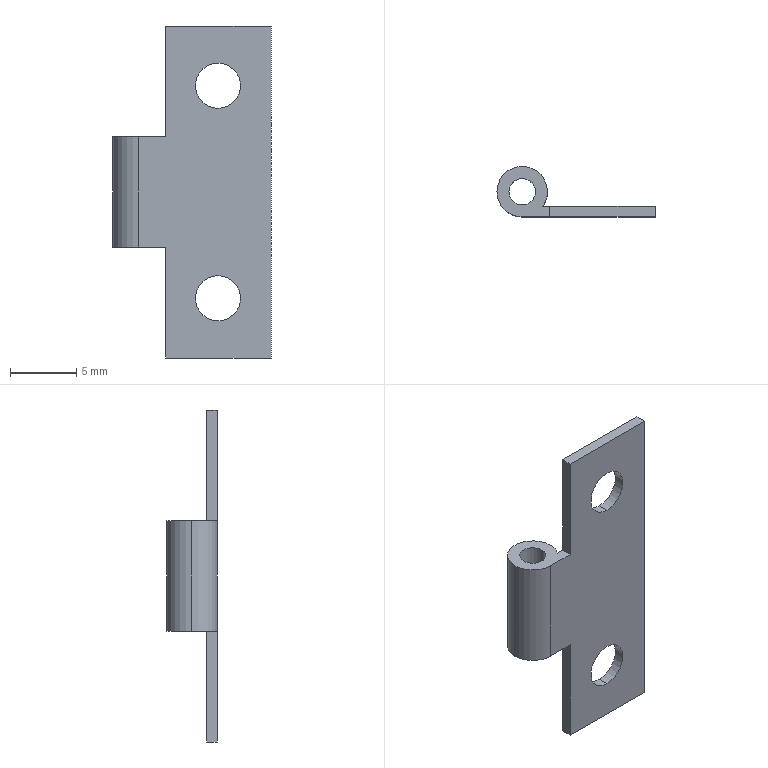Part | SolidWorks | features ICE 3, RefAxis 3, 3DProfileFeature 1, Extrusion 1 | 1 solid | 18 faces | box 11.9 x 3.8 x 25 mm | volume 218.697 mm3 | cylinder 9 | plane 9 | commonest cylinder face diameters 3.4 x4 3.8 x3 2 x2
STEP:
#1=CARTESIAN_POINT('',(6.,0.8,-6.2));
#2=VERTEX_POINT('',#1);
#3=CARTESIAN_POINT('',(6.,0.8,-2.8));
#4=VERTEX_POINT('',#3);
#5=CARTESIAN_POINT('',(6.,0.8,-4.5));
#6=DIRECTION('',(0.,1.,0.));
#7=DIRECTION('',(0.,0.,1.));
#8=AXIS2_PLACEMENT_3D('',#5,#6,#7);
#9=CIRCLE('',#8,1.7);
#10=EDGE_CURVE('',#2,#4,#9,.T.);
#11=ORIENTED_EDGE('',*,*,#10,.T.);
#12=CARTESIAN_POINT('',(6.,0.,-2.8));
#13=VERTEX_POINT('',#12);
#14=CARTESIAN_POINT('',(6.,0.8,-2.8));
#15=DIRECTION('',(0.,-1.,0.));
#16=VECTOR('',#15,1000.);
#17=LINE('',#14,#16);
#18=EDGE_CURVE('',#4,#13,#17,.T.);
#19=ORIENTED_EDGE('',*,*,#18,.T.);
#20=CARTESIAN_POINT('',(6.,0.,-6.2));
#21=VERTEX_POINT('',#20);
#22=CARTESIAN_POINT('',(6.,0.,-4.5));
#23=DIRECTION('',(0.,1.,0.));
#24=DIRECTION('',(0.,0.,1.));
#25=AXIS2_PLACEMENT_3D('',#22,#23,#24);
#26=CIRCLE('',#25,1.7);
#27=EDGE_CURVE('',#21,#13,#26,.T.);
#28=ORIENTED_EDGE('',*,*,#27,.F.);
#29=CARTESIAN_POINT('',(6.,0.8,-6.2));
#30=DIRECTION('',(0.,-1.,0.));
#31=VECTOR('',#30,1000.);
#32=LINE('',#29,#31);
#33=EDGE_CURVE('',#2,#21,#32,.T.);
#34=ORIENTED_EDGE('',*,*,#33,.F.);
#35=EDGE_LOOP('',(#11,#19,#28,#34));
#36=FACE_OUTER_BOUND('',#35,.T.);
#37=CARTESIAN_POINT('',(6.,0.8,-4.5));
#38=DIRECTION('',(0.,-1.,0.));
#39=DIRECTION('',(0.,0.,-1.));
#40=AXIS2_PLACEMENT_3D('',#37,#38,#39);
#41=CYLINDRICAL_SURFACE('',#40,1.7);
#42=ADVANCED_FACE('',(#36),#41,.F.);
#43=CARTESIAN_POINT('',(6.,0.8,-22.2));
#44=VERTEX_POINT('',#43);
#45=CARTESIAN_POINT('',(6.,0.8,-18.8));
#46=VERTEX_POINT('',#45);
#47=CARTESIAN_POINT('',(6.,0.8,-20.5));
#48=DIRECTION('',(0.,1.,0.));
#49=DIRECTION('',(0.,0.,1.));
#50=AXIS2_PLACEMENT_3D('',#47,#48,#49);
#51=CIRCLE('',#50,1.7);
#52=EDGE_CURVE('',#44,#46,#51,.T.);
#53=ORIENTED_EDGE('',*,*,#52,.T.);
#54=CARTESIAN_POINT('',(6.,0.,-18.8));
#55=VERTEX_POINT('',#54);
#56=CARTESIAN_POINT('',(6.,0.8,-18.8));
#57=DIRECTION('',(0.,-1.,0.));
#58=VECTOR('',#57,1000.);
#59=LINE('',#56,#58);
#60=EDGE_CURVE('',#46,#55,#59,.T.);
#61=ORIENTED_EDGE('',*,*,#60,.T.);
#62=CARTESIAN_POINT('',(6.,0.,-22.2));
#63=VERTEX_POINT('',#62);
#64=CARTESIAN_POINT('',(6.,0.,-20.5));
#65=DIRECTION('',(0.,1.,0.));
#66=DIRECTION('',(0.,0.,1.));
#67=AXIS2_PLACEMENT_3D('',#64,#65,#66);
#68=CIRCLE('',#67,1.7);
#69=EDGE_CURVE('',#63,#55,#68,.T.);
#70=ORIENTED_EDGE('',*,*,#69,.F.);
#71=CARTESIAN_POINT('',(6.,0.8,-22.2));
#72=DIRECTION('',(0.,-1.,0.));
#73=VECTOR('',#72,1000.);
#74=LINE('',#71,#73);
#75=EDGE_CURVE('',#44,#63,#74,.T.);
#76=ORIENTED_EDGE('',*,*,#75,.F.);
#77=EDGE_LOOP('',(#53,#61,#70,#76));
#78=FACE_OUTER_BOUND('',#77,.T.);
#79=CARTESIAN_POINT('',(6.,0.8,-20.5));
#80=DIRECTION('',(0.,-1.,0.));
#81=DIRECTION('',(0.,0.,-1.));
#82=AXIS2_PLACEMENT_3D('',#79,#80,#81);
#83=CYLINDRICAL_SURFACE('',#82,1.7);
#84=ADVANCED_FACE('',(#78),#83,.F.);
#85=CARTESIAN_POINT('',(-1.,1.9,-16.667));
#86=VERTEX_POINT('',#85);
#87=CARTESIAN_POINT('',(1.,1.9,-16.667));
#88=VERTEX_POINT('',#87);
#89=CARTESIAN_POINT('',(0.,1.9,-16.667));
#90=DIRECTION('',(0.,0.,1.));
#91=DIRECTION('',(-1.,0.,0.));
#92=AXIS2_PLACEMENT_3D('',#89,#90,#91);
#93=CIRCLE('',#92,1.);
#94=EDGE_CURVE('',#86,#88,#93,.T.);
#95=ORIENTED_EDGE('',*,*,#94,.F.);
#96=CARTESIAN_POINT('',(-1.,1.9,-8.333));
#97=VERTEX_POINT('',#96);
#98=CARTESIAN_POINT('',(-1.,1.9,-25.));
#99=DIRECTION('',(0.,0.,1.));
#100=VECTOR('',#99,1000.);
#101=LINE('',#98,#100);
#102=EDGE_CURVE('',#86,#97,#101,.T.);
#103=ORIENTED_EDGE('',*,*,#102,.T.);
#104=CARTESIAN_POINT('',(1.,1.9,-8.333));
#105=VERTEX_POINT('',#104);
#106=CARTESIAN_POINT('',(0.,1.9,-8.333));
#107=DIRECTION('',(0.,0.,-1.));
#108=DIRECTION('',(1.,0.,0.));
#109=AXIS2_PLACEMENT_3D('',#106,#107,#108);
#110=CIRCLE('',#109,1.);
#111=EDGE_CURVE('',#105,#97,#110,.T.);
#112=ORIENTED_EDGE('',*,*,#111,.F.);
#113=CARTESIAN_POINT('',(1.,1.9,-25.));
#114=DIRECTION('',(0.,0.,1.));
#115=VECTOR('',#114,1000.);
#116=LINE('',#113,#115);
#117=EDGE_CURVE('',#88,#105,#116,.T.);
#118=ORIENTED_EDGE('',*,*,#117,.F.);
#119=EDGE_LOOP('',(#95,#103,#112,#118));
#120=FACE_OUTER_BOUND('',#119,.T.);
#121=CARTESIAN_POINT('',(0.,1.9,-25.));
#122=DIRECTION('',(0.,0.,1.));
#123=DIRECTION('',(1.,0.,0.));
#124=AXIS2_PLACEMENT_3D('',#121,#122,#123);
#125=CYLINDRICAL_SURFACE('',#124,1.);
#126=ADVANCED_FACE('',(#120),#125,.F.);
#127=CARTESIAN_POINT('',(1.9,1.9,-16.667));
#128=VERTEX_POINT('',#127);
#129=CARTESIAN_POINT('',(-1.9,1.9,-16.667));
#130=VERTEX_POINT('',#129);
#131=CARTESIAN_POINT('',(0.,1.9,-16.667));
#132=DIRECTION('',(0.,0.,1.));
#133=DIRECTION('',(-1.,0.,0.));
#134=AXIS2_PLACEMENT_3D('',#131,#132,#133);
#135=CIRCLE('',#134,1.9);
#136=EDGE_CURVE('',#128,#130,#135,.T.);
#137=ORIENTED_EDGE('',*,*,#136,.T.);
#138=CARTESIAN_POINT('',(-1.9,1.9,-8.333));
#139=VERTEX_POINT('',#138);
#140=CARTESIAN_POINT('',(-1.9,1.9,-25.));
#141=DIRECTION('',(0.,0.,1.));
#142=VECTOR('',#141,1000.);
#143=LINE('',#140,#142);
#144=EDGE_CURVE('',#130,#139,#143,.T.);
#145=ORIENTED_EDGE('',*,*,#144,.T.);
#146=CARTESIAN_POINT('',(1.9,1.9,-8.333));
#147=VERTEX_POINT('',#146);
#148=CARTESIAN_POINT('',(0.,1.9,-8.333));
#149=DIRECTION('',(0.,0.,-1.));
#150=DIRECTION('',(1.,0.,0.));
#151=AXIS2_PLACEMENT_3D('',#148,#149,#150);
#152=CIRCLE('',#151,1.9);
#153=EDGE_CURVE('',#139,#147,#152,.T.);
#154=ORIENTED_EDGE('',*,*,#153,.T.);
#155=CARTESIAN_POINT('',(1.9,1.9,-25.));
#156=DIRECTION('',(0.,0.,1.));
#157=VECTOR('',#156,1000.);
#158=LINE('',#155,#157);
#159=EDGE_CURVE('',#128,#147,#158,.T.);
#160=ORIENTED_EDGE('',*,*,#159,.F.);
#161=EDGE_LOOP('',(#137,#145,#154,#160));
#162=FACE_OUTER_BOUND('',#161,.T.);
#163=CARTESIAN_POINT('',(0.,1.9,-25.));
#164=DIRECTION('',(0.,0.,1.));
#165=DIRECTION('',(1.,0.,0.));
#166=AXIS2_PLACEMENT_3D('',#163,#164,#165);
#167=CYLINDRICAL_SURFACE('',#166,1.9);
#168=ADVANCED_FACE('',(#162),#167,.T.);
#169=CARTESIAN_POINT('',(1.549,0.8,-16.667));
#170=VERTEX_POINT('',#169);
#171=CARTESIAN_POINT('',(0.,1.9,-16.667));
#172=DIRECTION('',(0.,0.,1.));
#173=DIRECTION('',(-1.,0.,0.));
#174=AXIS2_PLACEMENT_3D('',#171,#172,#173);
#175=CIRCLE('',#174,1.9);
#176=EDGE_CURVE('',#170,#128,#175,.T.);
#177=ORIENTED_EDGE('',*,*,#176,.T.);
#178=ORIENTED_EDGE('',*,*,#159,.T.);
#179=CARTESIAN_POINT('',(1.549,0.8,-8.333));
#180=VERTEX_POINT('',#179);
#181=CARTESIAN_POINT('',(0.,1.9,-8.333));
#182=DIRECTION('',(0.,0.,-1.));
#183=DIRECTION('',(1.,0.,0.));
#184=AXIS2_PLACEMENT_3D('',#181,#182,#183);
#185=CIRCLE('',#184,1.9);
#186=EDGE_CURVE('',#147,#180,#185,.T.);
#187=ORIENTED_EDGE('',*,*,#186,.T.);
#188=CARTESIAN_POINT('',(1.549,0.8,-25.));
#189=DIRECTION('',(0.,0.,1.));
#190=VECTOR('',#189,1000.);
#191=LINE('',#188,#190);
#192=EDGE_CURVE('',#170,#180,#191,.T.);
#193=ORIENTED_EDGE('',*,*,#192,.F.);
#194=EDGE_LOOP('',(#177,#178,#187,#193));
#195=FACE_OUTER_BOUND('',#194,.T.);
#196=CARTESIAN_POINT('',(0.,1.9,-25.));
#197=DIRECTION('',(0.,0.,1.));
#198=DIRECTION('',(1.,0.,0.));
#199=AXIS2_PLACEMENT_3D('',#196,#197,#198);
#200=CYLINDRICAL_SURFACE('',#199,1.9);
#201=ADVANCED_FACE('',(#195),#200,.T.);
#202=ORIENTED_EDGE('',*,*,#52,.F.);
#203=CARTESIAN_POINT('',(6.,0.8,-20.5));
#204=DIRECTION('',(0.,1.,0.));
#205=DIRECTION('',(0.,0.,1.));
#206=AXIS2_PLACEMENT_3D('',#203,#204,#205);
#207=CIRCLE('',#206,1.7);
#208=EDGE_CURVE('',#46,#44,#207,.T.);
#209=ORIENTED_EDGE('',*,*,#208,.F.);
#210=EDGE_LOOP('',(#202,#209));
#211=FACE_BOUND('',#210,.T.);
#212=CARTESIAN_POINT('',(2.09,0.8,-8.333));
#213=VERTEX_POINT('',#212);
#214=CARTESIAN_POINT('',(10.,0.8,-8.333));
#215=DIRECTION('',(1.,0.,0.));
#216=VECTOR('',#215,1000.);
#217=LINE('',#214,#216);
#218=EDGE_CURVE('',#180,#213,#217,.T.);
#219=ORIENTED_EDGE('',*,*,#218,.T.);
#220=CARTESIAN_POINT('',(2.09,0.8,0.));
#221=VERTEX_POINT('',#220);
#222=CARTESIAN_POINT('',(2.09,0.8,-25.));
#223=DIRECTION('',(0.,0.,1.));
#224=VECTOR('',#223,1000.);
#225=LINE('',#222,#224);
#226=EDGE_CURVE('',#213,#221,#225,.T.);
#227=ORIENTED_EDGE('',*,*,#226,.T.);
#228=CARTESIAN_POINT('',(10.,0.8,0.));
#229=VERTEX_POINT('',#228);
#230=CARTESIAN_POINT('',(10.,0.8,0.));
#231=DIRECTION('',(-1.,0.,0.));
#232=VECTOR('',#231,1000.);
#233=LINE('',#230,#232);
#234=EDGE_CURVE('',#229,#221,#233,.T.);
#235=ORIENTED_EDGE('',*,*,#234,.F.);
#236=CARTESIAN_POINT('',(10.,0.8,-25.));
#237=VERTEX_POINT('',#236);
#238=CARTESIAN_POINT('',(10.,0.8,-25.));
#239=DIRECTION('',(0.,0.,1.));
#240=VECTOR('',#239,1000.);
#241=LINE('',#238,#240);
#242=EDGE_CURVE('',#237,#229,#241,.T.);
#243=ORIENTED_EDGE('',*,*,#242,.F.);
#244=CARTESIAN_POINT('',(2.09,0.8,-25.));
#245=VERTEX_POINT('',#244);
#246=CARTESIAN_POINT('',(10.,0.8,-25.));
#247=DIRECTION('',(-1.,0.,0.));
#248=VECTOR('',#247,1000.);
#249=LINE('',#246,#248);
#250=EDGE_CURVE('',#237,#245,#249,.T.);
#251=ORIENTED_EDGE('',*,*,#250,.T.);
#252=CARTESIAN_POINT('',(2.09,0.8,-16.667));
#253=VERTEX_POINT('',#252);
#254=CARTESIAN_POINT('',(2.09,0.8,-25.));
#255=DIRECTION('',(0.,0.,1.));
#256=VECTOR('',#255,1000.);
#257=LINE('',#254,#256);
#258=EDGE_CURVE('',#245,#253,#257,.T.);
#259=ORIENTED_EDGE('',*,*,#258,.T.);
#260=CARTESIAN_POINT('',(10.,0.8,-16.667));
#261=DIRECTION('',(-1.,0.,0.));
#262=VECTOR('',#261,1000.);
#263=LINE('',#260,#262);
#264=EDGE_CURVE('',#253,#170,#263,.T.);
#265=ORIENTED_EDGE('',*,*,#264,.T.);
#266=ORIENTED_EDGE('',*,*,#192,.T.);
#267=EDGE_LOOP('',(#219,#227,#235,#243,#251,#259,#265,#266));
#268=FACE_OUTER_BOUND('',#267,.T.);
#269=ORIENTED_EDGE('',*,*,#10,.F.);
#270=CARTESIAN_POINT('',(6.,0.8,-4.5));
#271=DIRECTION('',(0.,1.,0.));
#272=DIRECTION('',(0.,0.,1.));
#273=AXIS2_PLACEMENT_3D('',#270,#271,#272);
#274=CIRCLE('',#273,1.7);
#275=EDGE_CURVE('',#4,#2,#274,.T.);
#276=ORIENTED_EDGE('',*,*,#275,.F.);
#277=EDGE_LOOP('',(#269,#276));
#278=FACE_BOUND('',#277,.T.);
#279=CARTESIAN_POINT('',(10.,0.8,-25.));
#280=DIRECTION('',(0.,1.,0.));
#281=DIRECTION('',(0.,0.,1.));
#282=AXIS2_PLACEMENT_3D('',#279,#280,#281);
#283=PLANE('',#282);
#284=ADVANCED_FACE('',(#211,#268,#278),#283,.T.);
#285=ORIENTED_EDGE('',*,*,#69,.T.);
#286=CARTESIAN_POINT('',(6.,0.,-20.5));
#287=DIRECTION('',(0.,1.,0.));
#288=DIRECTION('',(0.,0.,1.));
#289=AXIS2_PLACEMENT_3D('',#286,#287,#288);
#290=CIRCLE('',#289,1.7);
#291=EDGE_CURVE('',#55,#63,#290,.T.);
#292=ORIENTED_EDGE('',*,*,#291,.T.);
#293=EDGE_LOOP('',(#285,#292));
#294=FACE_BOUND('',#293,.T.);
#295=CARTESIAN_POINT('',(2.09,0.,0.));
#296=VERTEX_POINT('',#295);
#297=CARTESIAN_POINT('',(10.,0.,0.));
#298=VERTEX_POINT('',#297);
#299=CARTESIAN_POINT('',(0.,0.,0.));
#300=DIRECTION('',(1.,0.,0.));
#301=VECTOR('',#300,1000.);
#302=LINE('',#299,#301);
#303=EDGE_CURVE('',#296,#298,#302,.T.);
#304=ORIENTED_EDGE('',*,*,#303,.F.);
#305=CARTESIAN_POINT('',(2.09,0.,-8.333));
#306=VERTEX_POINT('',#305);
#307=CARTESIAN_POINT('',(2.09,0.,0.));
#308=DIRECTION('',(0.,0.,-1.));
#309=VECTOR('',#308,1000.);
#310=LINE('',#307,#309);
#311=EDGE_CURVE('',#296,#306,#310,.T.);
#312=ORIENTED_EDGE('',*,*,#311,.T.);
#313=CARTESIAN_POINT('',(0.,0.,-8.333));
#314=VERTEX_POINT('',#313);
#315=CARTESIAN_POINT('',(2.09,0.,-8.333));
#316=DIRECTION('',(-1.,0.,0.));
#317=VECTOR('',#316,1000.);
#318=LINE('',#315,#317);
#319=EDGE_CURVE('',#306,#314,#318,.T.);
#320=ORIENTED_EDGE('',*,*,#319,.T.);
#321=CARTESIAN_POINT('',(0.,0.,-16.667));
#322=VERTEX_POINT('',#321);
#323=CARTESIAN_POINT('',(0.,0.,-25.));
#324=DIRECTION('',(0.,0.,1.));
#325=VECTOR('',#324,1000.);
#326=LINE('',#323,#325);
#327=EDGE_CURVE('',#322,#314,#326,.T.);
#328=ORIENTED_EDGE('',*,*,#327,.F.);
#329=CARTESIAN_POINT('',(2.09,0.,-16.667));
#330=VERTEX_POINT('',#329);
#331=CARTESIAN_POINT('',(-2.09,0.,-16.667));
#332=DIRECTION('',(1.,0.,0.));
#333=VECTOR('',#332,1000.);
#334=LINE('',#331,#333);
#335=EDGE_CURVE('',#322,#330,#334,.T.);
#336=ORIENTED_EDGE('',*,*,#335,.T.);
#337=CARTESIAN_POINT('',(2.09,0.,-25.));
#338=VERTEX_POINT('',#337);
#339=CARTESIAN_POINT('',(2.09,0.,-16.667));
#340=DIRECTION('',(0.,0.,-1.));
#341=VECTOR('',#340,1000.);
#342=LINE('',#339,#341);
#343=EDGE_CURVE('',#330,#338,#342,.T.);
#344=ORIENTED_EDGE('',*,*,#343,.T.);
#345=CARTESIAN_POINT('',(10.,0.,-25.));
#346=VERTEX_POINT('',#345);
#347=CARTESIAN_POINT('',(0.,0.,-25.));
#348=DIRECTION('',(1.,0.,0.));
#349=VECTOR('',#348,1000.);
#350=LINE('',#347,#349);
#351=EDGE_CURVE('',#338,#346,#350,.T.);
#352=ORIENTED_EDGE('',*,*,#351,.T.);
#353=CARTESIAN_POINT('',(10.,0.,-25.));
#354=DIRECTION('',(0.,0.,1.));
#355=VECTOR('',#354,1000.);
#356=LINE('',#353,#355);
#357=EDGE_CURVE('',#346,#298,#356,.T.);
#358=ORIENTED_EDGE('',*,*,#357,.T.);
#359=EDGE_LOOP('',(#304,#312,#320,#328,#336,#344,#352,#358));
#360=FACE_OUTER_BOUND('',#359,.T.);
#361=ORIENTED_EDGE('',*,*,#27,.T.);
#362=CARTESIAN_POINT('',(6.,0.,-4.5));
#363=DIRECTION('',(0.,1.,0.));
#364=DIRECTION('',(0.,0.,1.));
#365=AXIS2_PLACEMENT_3D('',#362,#363,#364);
#366=CIRCLE('',#365,1.7);
#367=EDGE_CURVE('',#13,#21,#366,.T.);
#368=ORIENTED_EDGE('',*,*,#367,.T.);
#369=EDGE_LOOP('',(#361,#368));
#370=FACE_BOUND('',#369,.T.);
#371=CARTESIAN_POINT('',(0.,0.,-25.));
#372=DIRECTION('',(0.,-1.,0.));
#373=DIRECTION('',(0.,0.,-1.));
#374=AXIS2_PLACEMENT_3D('',#371,#372,#373);
#375=PLANE('',#374);
#376=ADVANCED_FACE('',(#294,#360,#370),#375,.T.);
#377=ORIENTED_EDGE('',*,*,#144,.F.);
#378=CARTESIAN_POINT('',(0.,1.9,-16.667));
#379=DIRECTION('',(0.,0.,1.));
#380=DIRECTION('',(-1.,0.,0.));
#381=AXIS2_PLACEMENT_3D('',#378,#379,#380);
#382=CIRCLE('',#381,1.9);
#383=EDGE_CURVE('',#130,#322,#382,.T.);
#384=ORIENTED_EDGE('',*,*,#383,.T.);
#385=ORIENTED_EDGE('',*,*,#327,.T.);
#386=CARTESIAN_POINT('',(0.,1.9,-8.333));
#387=DIRECTION('',(0.,0.,-1.));
#388=DIRECTION('',(1.,0.,0.));
#389=AXIS2_PLACEMENT_3D('',#386,#387,#388);
#390=CIRCLE('',#389,1.9);
#391=EDGE_CURVE('',#314,#139,#390,.T.);
#392=ORIENTED_EDGE('',*,*,#391,.T.);
#393=EDGE_LOOP('',(#377,#384,#385,#392));
#394=FACE_OUTER_BOUND('',#393,.T.);
#395=CARTESIAN_POINT('',(0.,1.9,-25.));
#396=DIRECTION('',(0.,0.,1.));
#397=DIRECTION('',(1.,0.,0.));
#398=AXIS2_PLACEMENT_3D('',#395,#396,#397);
#399=CYLINDRICAL_SURFACE('',#398,1.9);
#400=ADVANCED_FACE('',(#394),#399,.T.);
#401=CARTESIAN_POINT('',(2.09,3.8,-25.));
#402=DIRECTION('',(0.,-1.,0.));
#403=VECTOR('',#402,1000.);
#404=LINE('',#401,#403);
#405=EDGE_CURVE('',#245,#338,#404,.T.);
#406=ORIENTED_EDGE('',*,*,#405,.F.);
#407=ORIENTED_EDGE('',*,*,#250,.F.);
#408=CARTESIAN_POINT('',(10.,0.,-25.));
#409=DIRECTION('',(0.,1.,0.));
#410=VECTOR('',#409,1000.);
#411=LINE('',#408,#410);
#412=EDGE_CURVE('',#346,#237,#411,.T.);
#413=ORIENTED_EDGE('',*,*,#412,.F.);
#414=ORIENTED_EDGE('',*,*,#351,.F.);
#415=EDGE_LOOP('',(#406,#407,#413,#414));
#416=FACE_OUTER_BOUND('',#415,.T.);
#417=CARTESIAN_POINT('',(0.,1.9,-25.));
#418=DIRECTION('',(0.,0.,1.));
#419=DIRECTION('',(1.,0.,0.));
#420=AXIS2_PLACEMENT_3D('',#417,#418,#419);
#421=PLANE('',#420);
#422=ADVANCED_FACE('',(#416),#421,.F.);
#423=ORIENTED_EDGE('',*,*,#234,.T.);
#424=CARTESIAN_POINT('',(2.09,3.8,0.));
#425=DIRECTION('',(0.,-1.,0.));
#426=VECTOR('',#425,1000.);
#427=LINE('',#424,#426);
#428=EDGE_CURVE('',#221,#296,#427,.T.);
#429=ORIENTED_EDGE('',*,*,#428,.T.);
#430=ORIENTED_EDGE('',*,*,#303,.T.);
#431=CARTESIAN_POINT('',(10.,0.,0.));
#432=DIRECTION('',(0.,1.,0.));
#433=VECTOR('',#432,1000.);
#434=LINE('',#431,#433);
#435=EDGE_CURVE('',#298,#229,#434,.T.);
#436=ORIENTED_EDGE('',*,*,#435,.T.);
#437=EDGE_LOOP('',(#423,#429,#430,#436));
#438=FACE_OUTER_BOUND('',#437,.T.);
#439=CARTESIAN_POINT('',(0.,1.9,0.));
#440=DIRECTION('',(0.,0.,1.));
#441=DIRECTION('',(1.,0.,0.));
#442=AXIS2_PLACEMENT_3D('',#439,#440,#441);
#443=PLANE('',#442);
#444=ADVANCED_FACE('',(#438),#443,.T.);
#445=ORIENTED_EDGE('',*,*,#435,.F.);
#446=ORIENTED_EDGE('',*,*,#357,.F.);
#447=ORIENTED_EDGE('',*,*,#412,.T.);
#448=ORIENTED_EDGE('',*,*,#242,.T.);
#449=EDGE_LOOP('',(#445,#446,#447,#448));
#450=FACE_OUTER_BOUND('',#449,.T.);
#451=CARTESIAN_POINT('',(10.,0.,-25.));
#452=DIRECTION('',(1.,0.,0.));
#453=DIRECTION('',(0.,0.,-1.));
#454=AXIS2_PLACEMENT_3D('',#451,#452,#453);
#455=PLANE('',#454);
#456=ADVANCED_FACE('',(#450),#455,.T.);
#457=ORIENTED_EDGE('',*,*,#176,.F.);
#458=ORIENTED_EDGE('',*,*,#264,.F.);
#459=CARTESIAN_POINT('',(2.09,3.8,-16.667));
#460=DIRECTION('',(0.,-1.,0.));
#461=VECTOR('',#460,1000.);
#462=LINE('',#459,#461);
#463=EDGE_CURVE('',#253,#330,#462,.T.);
#464=ORIENTED_EDGE('',*,*,#463,.T.);
#465=ORIENTED_EDGE('',*,*,#335,.F.);
#466=ORIENTED_EDGE('',*,*,#383,.F.);
#467=ORIENTED_EDGE('',*,*,#136,.F.);
#468=EDGE_LOOP('',(#457,#458,#464,#465,#466,#467));
#469=FACE_OUTER_BOUND('',#468,.T.);
#470=CARTESIAN_POINT('',(0.,1.9,-16.667));
#471=DIRECTION('',(0.,0.,1.));
#472=DIRECTION('',(-1.,0.,0.));
#473=AXIS2_PLACEMENT_3D('',#470,#471,#472);
#474=CIRCLE('',#473,1.);
#475=EDGE_CURVE('',#88,#86,#474,.T.);
#476=ORIENTED_EDGE('',*,*,#475,.T.);
#477=ORIENTED_EDGE('',*,*,#94,.T.);
#478=EDGE_LOOP('',(#476,#477));
#479=FACE_BOUND('',#478,.T.);
#480=CARTESIAN_POINT('',(-2.09,3.8,-16.667));
#481=DIRECTION('',(0.,0.,-1.));
#482=DIRECTION('',(-1.,0.,0.));
#483=AXIS2_PLACEMENT_3D('',#480,#481,#482);
#484=PLANE('',#483);
#485=ADVANCED_FACE('',(#469,#479),#484,.T.);
#486=ORIENTED_EDGE('',*,*,#405,.T.);
#487=ORIENTED_EDGE('',*,*,#343,.F.);
#488=ORIENTED_EDGE('',*,*,#463,.F.);
#489=ORIENTED_EDGE('',*,*,#258,.F.);
#490=EDGE_LOOP('',(#486,#487,#488,#489));
#491=FACE_OUTER_BOUND('',#490,.T.);
#492=CARTESIAN_POINT('',(2.09,3.8,-16.667));
#493=DIRECTION('',(-1.,0.,0.));
#494=DIRECTION('',(0.,0.,1.));
#495=AXIS2_PLACEMENT_3D('',#492,#493,#494);
#496=PLANE('',#495);
#497=ADVANCED_FACE('',(#491),#496,.T.);
#498=ORIENTED_EDGE('',*,*,#319,.F.);
#499=CARTESIAN_POINT('',(2.09,3.8,-8.333));
#500=DIRECTION('',(0.,-1.,0.));
#501=VECTOR('',#500,1000.);
#502=LINE('',#499,#501);
#503=EDGE_CURVE('',#213,#306,#502,.T.);
#504=ORIENTED_EDGE('',*,*,#503,.F.);
#505=ORIENTED_EDGE('',*,*,#218,.F.);
#506=ORIENTED_EDGE('',*,*,#186,.F.);
#507=ORIENTED_EDGE('',*,*,#153,.F.);
#508=ORIENTED_EDGE('',*,*,#391,.F.);
#509=EDGE_LOOP('',(#498,#504,#505,#506,#507,#508));
#510=FACE_OUTER_BOUND('',#509,.T.);
#511=ORIENTED_EDGE('',*,*,#111,.T.);
#512=CARTESIAN_POINT('',(0.,1.9,-8.333));
#513=DIRECTION('',(0.,0.,-1.));
#514=DIRECTION('',(1.,0.,0.));
#515=AXIS2_PLACEMENT_3D('',#512,#513,#514);
#516=CIRCLE('',#515,1.);
#517=EDGE_CURVE('',#97,#105,#516,.T.);
#518=ORIENTED_EDGE('',*,*,#517,.T.);
#519=EDGE_LOOP('',(#511,#518));
#520=FACE_BOUND('',#519,.T.);
#521=CARTESIAN_POINT('',(2.09,3.8,-8.333));
#522=DIRECTION('',(0.,0.,1.));
#523=DIRECTION('',(1.,0.,0.));
#524=AXIS2_PLACEMENT_3D('',#521,#522,#523);
#525=PLANE('',#524);
#526=ADVANCED_FACE('',(#510,#520),#525,.T.);
#527=ORIENTED_EDGE('',*,*,#503,.T.);
#528=ORIENTED_EDGE('',*,*,#311,.F.);
#529=ORIENTED_EDGE('',*,*,#428,.F.);
#530=ORIENTED_EDGE('',*,*,#226,.F.);
#531=EDGE_LOOP('',(#527,#528,#529,#530));
#532=FACE_OUTER_BOUND('',#531,.T.);
#533=CARTESIAN_POINT('',(2.09,3.8,0.));
#534=DIRECTION('',(-1.,0.,0.));
#535=DIRECTION('',(0.,0.,1.));
#536=AXIS2_PLACEMENT_3D('',#533,#534,#535);
#537=PLANE('',#536);
#538=ADVANCED_FACE('',(#532),#537,.T.);
#539=ORIENTED_EDGE('',*,*,#102,.F.);
#540=ORIENTED_EDGE('',*,*,#475,.F.);
#541=ORIENTED_EDGE('',*,*,#117,.T.);
#542=ORIENTED_EDGE('',*,*,#517,.F.);
#543=EDGE_LOOP('',(#539,#540,#541,#542));
#544=FACE_OUTER_BOUND('',#543,.T.);
#545=CARTESIAN_POINT('',(0.,1.9,-25.));
#546=DIRECTION('',(0.,0.,1.));
#547=DIRECTION('',(1.,0.,0.));
#548=AXIS2_PLACEMENT_3D('',#545,#546,#547);
#549=CYLINDRICAL_SURFACE('',#548,1.);
#550=ADVANCED_FACE('',(#544),#549,.F.);
#551=ORIENTED_EDGE('',*,*,#60,.F.);
#552=ORIENTED_EDGE('',*,*,#208,.T.);
#553=ORIENTED_EDGE('',*,*,#75,.T.);
#554=ORIENTED_EDGE('',*,*,#291,.F.);
#555=EDGE_LOOP('',(#551,#552,#553,#554));
#556=FACE_OUTER_BOUND('',#555,.T.);
#557=CARTESIAN_POINT('',(6.,0.8,-20.5));
#558=DIRECTION('',(0.,-1.,0.));
#559=DIRECTION('',(0.,0.,-1.));
#560=AXIS2_PLACEMENT_3D('',#557,#558,#559);
#561=CYLINDRICAL_SURFACE('',#560,1.7);
#562=ADVANCED_FACE('',(#556),#561,.F.);
#563=ORIENTED_EDGE('',*,*,#18,.F.);
#564=ORIENTED_EDGE('',*,*,#275,.T.);
#565=ORIENTED_EDGE('',*,*,#33,.T.);
#566=ORIENTED_EDGE('',*,*,#367,.F.);
#567=EDGE_LOOP('',(#563,#564,#565,#566));
#568=FACE_OUTER_BOUND('',#567,.T.);
#569=CARTESIAN_POINT('',(6.,0.8,-4.5));
#570=DIRECTION('',(0.,-1.,0.));
#571=DIRECTION('',(0.,0.,-1.));
#572=AXIS2_PLACEMENT_3D('',#569,#570,#571);
#573=CYLINDRICAL_SURFACE('',#572,1.7);
#574=ADVANCED_FACE('',(#568),#573,.F.);
#575=CLOSED_SHELL('',(#42,#84,#126,#168,#201,#284,#376,#400,#422,#444,#456,#485,#497,#526,#538,#550,#562,#574));
#576=MANIFOLD_SOLID_BREP('',#575);
#577=CARTESIAN_POINT('',(0.,0.,0.));
#578=DIRECTION('',(0.,0.,1.));
#579=DIRECTION('',(1.,0.,0.));
#580=AXIS2_PLACEMENT_3D('',#577,#578,#579);
#581=(LENGTH_UNIT()NAMED_UNIT(*)SI_UNIT(.MILLI.,.METRE.));
#582=UNCERTAINTY_MEASURE_WITH_UNIT(LENGTH_MEASURE(0.00001),#581,'','');
#583=(NAMED_UNIT(*)PLANE_ANGLE_UNIT()SI_UNIT($,.RADIAN.));
#584=(NAMED_UNIT(*)SI_UNIT($,.STERADIAN.)SOLID_ANGLE_UNIT());
#585=(GEOMETRIC_REPRESENTATION_CONTEXT(3)GLOBAL_UNCERTAINTY_ASSIGNED_CONTEXT((#582))GLOBAL_UNIT_ASSIGNED_CONTEXT((#581,#583,#584))REPRESENTATION_CONTEXT('',''));
#586=ADVANCED_BREP_SHAPE_REPRESENTATION('',(#576,#580),#585);